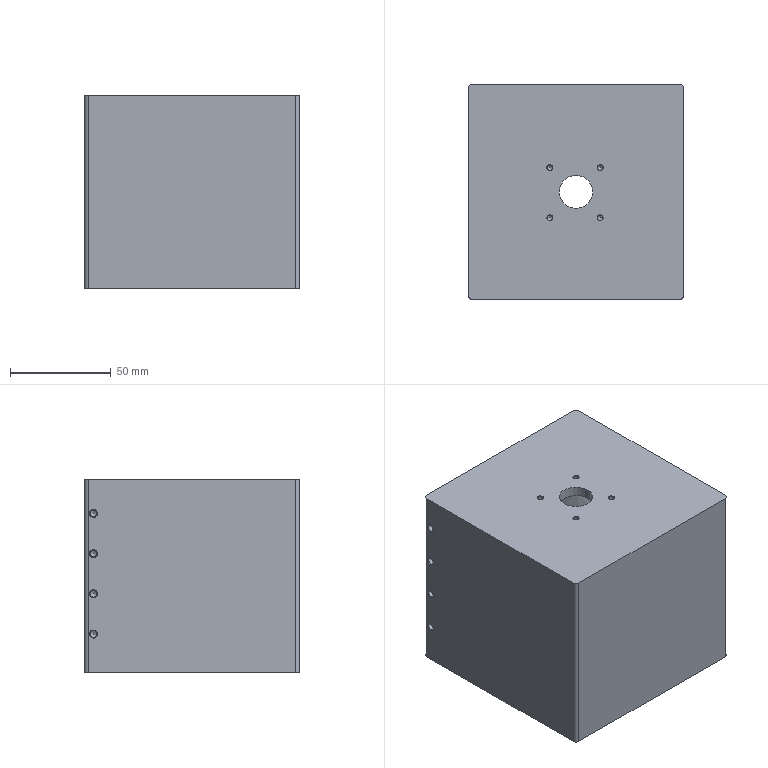Part | STEP file | Radial combiner outer cavity | 1 solid | 115 faces | box 107 x 107 x 96.43 mm | volume 625151 mm3 | cone 69 | cylinder 40 | plane 6 | commonest cylinder face diameters 3.3 x18 2.05 x12 2.5 x4 4 x4 16.5 x1 96.34 x1